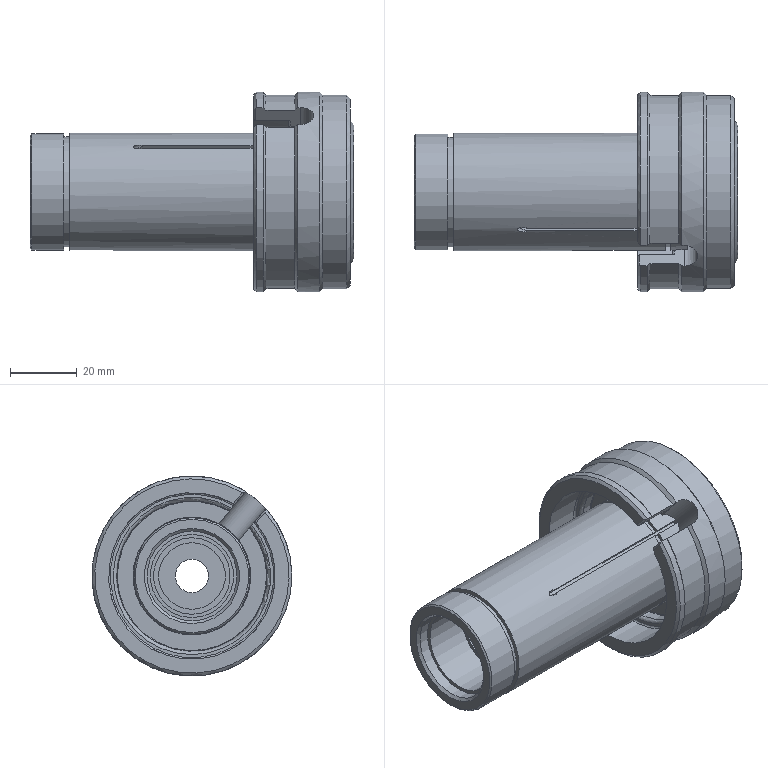Part | STEP file | Nozzle Body-2(02) | 1 solid | 57 faces | box 97 x 60 x 60 mm | volume 109750 mm3 | plane 23 | cylinder 20 | cone 10 | torus 4 | commonest cylinder face diameters 35.3 x2 58 x2 60 x2 1 x1 1.7 x1 8 x1